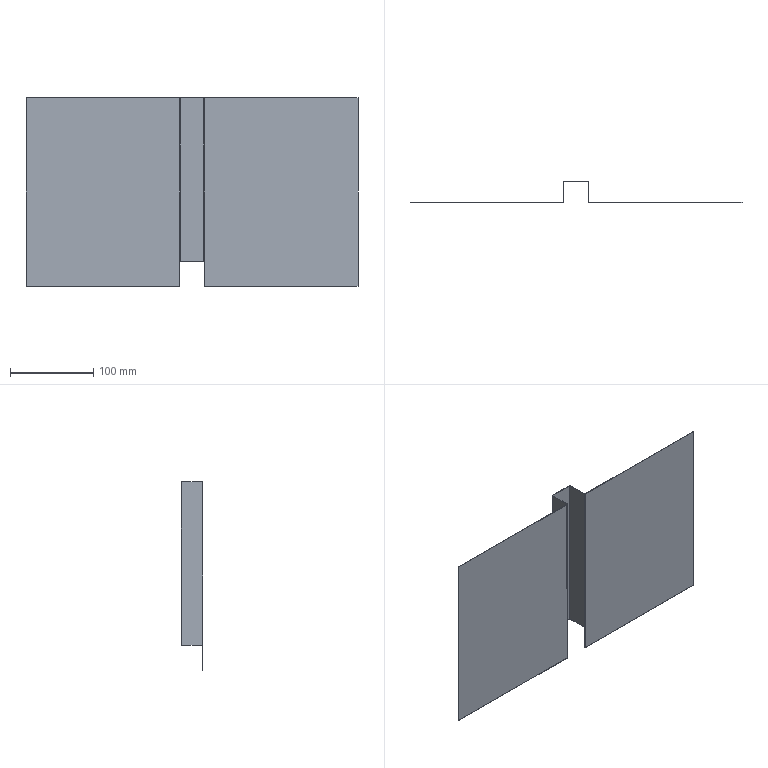Part | SolidWorks | features FlatPattern 1, ICE 1, SMBaseFlange 1, SheetMetal 1 | 1 solid | 36 faces | box 399 x 26 x 226 mm | volume 49527 mm3 | plane 28 | cylinder 8 | commonest cylinder face diameters 0.8 x4 1.8 x4
STEP:
#1=CARTESIAN_POINT('',(184.5,0.4,226.));
#2=VERTEX_POINT('',#1);
#3=CARTESIAN_POINT('',(185.,0.4,226.));
#4=VERTEX_POINT('',#3);
#5=CARTESIAN_POINT('',(184.5,0.4,226.));
#6=DIRECTION('',(1.,0.,0.));
#7=VECTOR('',#6,1000.);
#8=LINE('',#5,#7);
#9=EDGE_CURVE('',#2,#4,#8,.T.);
#10=ORIENTED_EDGE('',*,*,#9,.F.);
#11=CARTESIAN_POINT('',(184.1,0.,226.));
#12=VERTEX_POINT('',#11);
#13=CARTESIAN_POINT('',(184.1,0.4,226.));
#14=DIRECTION('',(0.,0.,1.));
#15=DIRECTION('',(-1.,0.,0.));
#16=AXIS2_PLACEMENT_3D('',#13,#14,#15);
#17=CIRCLE('',#16,0.4);
#18=EDGE_CURVE('',#12,#2,#17,.T.);
#19=ORIENTED_EDGE('',*,*,#18,.F.);
#20=CARTESIAN_POINT('',(184.1,-0.5,226.));
#21=VERTEX_POINT('',#20);
#22=CARTESIAN_POINT('',(184.1,-0.5,226.));
#23=DIRECTION('',(0.,1.,0.));
#24=VECTOR('',#23,1000.);
#25=LINE('',#22,#24);
#26=EDGE_CURVE('',#21,#12,#25,.T.);
#27=ORIENTED_EDGE('',*,*,#26,.F.);
#28=CARTESIAN_POINT('',(184.1,0.4,226.));
#29=DIRECTION('',(0.,0.,1.));
#30=DIRECTION('',(1.,0.,0.));
#31=AXIS2_PLACEMENT_3D('',#28,#29,#30);
#32=CIRCLE('',#31,0.9);
#33=EDGE_CURVE('',#21,#4,#32,.T.);
#34=ORIENTED_EDGE('',*,*,#33,.T.);
#35=EDGE_LOOP('',(#10,#19,#27,#34));
#36=FACE_OUTER_BOUND('',#35,.T.);
#37=CARTESIAN_POINT('',(184.5,0.4,226.));
#38=DIRECTION('',(0.,0.,1.));
#39=DIRECTION('',(1.,0.,0.));
#40=AXIS2_PLACEMENT_3D('',#37,#38,#39);
#41=PLANE('',#40);
#42=ADVANCED_FACE('',(#36),#41,.T.);
#43=CARTESIAN_POINT('',(184.5,24.6,226.));
#44=VERTEX_POINT('',#43);
#45=CARTESIAN_POINT('',(184.5,0.,226.));
#46=DIRECTION('',(0.,1.,0.));
#47=VECTOR('',#46,1000.);
#48=LINE('',#45,#47);
#49=EDGE_CURVE('',#2,#44,#48,.T.);
#50=ORIENTED_EDGE('',*,*,#49,.F.);
#51=ORIENTED_EDGE('',*,*,#9,.T.);
#52=CARTESIAN_POINT('',(185.,24.6,226.));
#53=VERTEX_POINT('',#52);
#54=CARTESIAN_POINT('',(185.,0.,226.));
#55=DIRECTION('',(0.,1.,0.));
#56=VECTOR('',#55,1000.);
#57=LINE('',#54,#56);
#58=EDGE_CURVE('',#4,#53,#57,.T.);
#59=ORIENTED_EDGE('',*,*,#58,.T.);
#60=CARTESIAN_POINT('',(185.,24.6,226.));
#61=DIRECTION('',(-1.,0.,0.));
#62=VECTOR('',#61,1000.);
#63=LINE('',#60,#62);
#64=EDGE_CURVE('',#53,#44,#63,.T.);
#65=ORIENTED_EDGE('',*,*,#64,.T.);
#66=EDGE_LOOP('',(#50,#51,#59,#65));
#67=FACE_OUTER_BOUND('',#66,.T.);
#68=CARTESIAN_POINT('',(184.1,-0.5,226.));
#69=DIRECTION('',(0.,0.,1.));
#70=DIRECTION('',(1.,0.,0.));
#71=AXIS2_PLACEMENT_3D('',#68,#69,#70);
#72=PLANE('',#71);
#73=ADVANCED_FACE('',(#67),#72,.T.);
#74=CARTESIAN_POINT('',(184.5,-0.4062,0.));
#75=VERTEX_POINT('',#74);
#76=CARTESIAN_POINT('',(184.5,0.4,0.));
#77=VERTEX_POINT('',#76);
#78=CARTESIAN_POINT('',(184.5,-0.501,0.));
#79=DIRECTION('',(0.,1.,0.));
#80=VECTOR('',#79,1000.);
#81=LINE('',#78,#80);
#82=EDGE_CURVE('',#75,#77,#81,.T.);
#83=ORIENTED_EDGE('',*,*,#82,.F.);
#84=CARTESIAN_POINT('',(184.1,-0.5,0.));
#85=VERTEX_POINT('',#84);
#86=CARTESIAN_POINT('',(184.1,0.4,0.));
#87=DIRECTION('',(0.,0.,1.));
#88=DIRECTION('',(1.,0.,0.));
#89=AXIS2_PLACEMENT_3D('',#86,#87,#88);
#90=CIRCLE('',#89,0.9);
#91=EDGE_CURVE('',#85,#75,#90,.T.);
#92=ORIENTED_EDGE('',*,*,#91,.F.);
#93=CARTESIAN_POINT('',(184.1,0.,0.));
#94=VERTEX_POINT('',#93);
#95=CARTESIAN_POINT('',(184.1,0.,0.));
#96=DIRECTION('',(0.,-1.,0.));
#97=VECTOR('',#96,1000.);
#98=LINE('',#95,#97);
#99=EDGE_CURVE('',#94,#85,#98,.T.);
#100=ORIENTED_EDGE('',*,*,#99,.F.);
#101=CARTESIAN_POINT('',(184.1,0.4,0.));
#102=DIRECTION('',(0.,0.,1.));
#103=DIRECTION('',(-1.,0.,0.));
#104=AXIS2_PLACEMENT_3D('',#101,#102,#103);
#105=CIRCLE('',#104,0.4);
#106=EDGE_CURVE('',#94,#77,#105,.T.);
#107=ORIENTED_EDGE('',*,*,#106,.T.);
#108=EDGE_LOOP('',(#83,#92,#100,#107));
#109=FACE_OUTER_BOUND('',#108,.T.);
#110=CARTESIAN_POINT('',(184.1,0.,0.));
#111=DIRECTION('',(0.,0.,-1.));
#112=DIRECTION('',(-1.,0.,0.));
#113=AXIS2_PLACEMENT_3D('',#110,#111,#112);
#114=PLANE('',#113);
#115=ADVANCED_FACE('',(#109),#114,.T.);
#116=CARTESIAN_POINT('',(0.,0.,0.));
#117=VERTEX_POINT('',#116);
#118=CARTESIAN_POINT('',(0.,0.,0.));
#119=DIRECTION('',(1.,0.,0.));
#120=VECTOR('',#119,1000.);
#121=LINE('',#118,#120);
#122=EDGE_CURVE('',#117,#94,#121,.T.);
#123=ORIENTED_EDGE('',*,*,#122,.T.);
#124=ORIENTED_EDGE('',*,*,#99,.T.);
#125=CARTESIAN_POINT('',(0.,-0.5,0.));
#126=VERTEX_POINT('',#125);
#127=CARTESIAN_POINT('',(0.,-0.5,0.));
#128=DIRECTION('',(1.,0.,0.));
#129=VECTOR('',#128,1000.);
#130=LINE('',#127,#129);
#131=EDGE_CURVE('',#126,#85,#130,.T.);
#132=ORIENTED_EDGE('',*,*,#131,.F.);
#133=CARTESIAN_POINT('',(0.,-0.5,0.));
#134=DIRECTION('',(0.,1.,0.));
#135=VECTOR('',#134,1000.);
#136=LINE('',#133,#135);
#137=EDGE_CURVE('',#126,#117,#136,.T.);
#138=ORIENTED_EDGE('',*,*,#137,.T.);
#139=EDGE_LOOP('',(#123,#124,#132,#138));
#140=FACE_OUTER_BOUND('',#139,.T.);
#141=CARTESIAN_POINT('',(185.,0.4,0.));
#142=DIRECTION('',(0.,0.,-1.));
#143=DIRECTION('',(-1.,0.,0.));
#144=AXIS2_PLACEMENT_3D('',#141,#142,#143);
#145=PLANE('',#144);
#146=ADVANCED_FACE('',(#140),#145,.T.);
#147=CARTESIAN_POINT('',(185.4,25.5,226.));
#148=VERTEX_POINT('',#147);
#149=CARTESIAN_POINT('',(185.4,25.,226.));
#150=VERTEX_POINT('',#149);
#151=CARTESIAN_POINT('',(185.4,25.5,226.));
#152=DIRECTION('',(0.,-1.,0.));
#153=VECTOR('',#152,1000.);
#154=LINE('',#151,#153);
#155=EDGE_CURVE('',#148,#150,#154,.T.);
#156=ORIENTED_EDGE('',*,*,#155,.F.);
#157=CARTESIAN_POINT('',(185.4,24.6,226.));
#158=DIRECTION('',(0.,0.,-1.));
#159=DIRECTION('',(1.,0.,0.));
#160=AXIS2_PLACEMENT_3D('',#157,#158,#159);
#161=CIRCLE('',#160,0.9);
#162=EDGE_CURVE('',#44,#148,#161,.T.);
#163=ORIENTED_EDGE('',*,*,#162,.F.);
#164=ORIENTED_EDGE('',*,*,#64,.F.);
#165=CARTESIAN_POINT('',(185.4,24.6,226.));
#166=DIRECTION('',(0.,0.,-1.));
#167=DIRECTION('',(1.,0.,0.));
#168=AXIS2_PLACEMENT_3D('',#165,#166,#167);
#169=CIRCLE('',#168,0.4);
#170=EDGE_CURVE('',#53,#150,#169,.T.);
#171=ORIENTED_EDGE('',*,*,#170,.T.);
#172=EDGE_LOOP('',(#156,#163,#164,#171));
#173=FACE_OUTER_BOUND('',#172,.T.);
#174=CARTESIAN_POINT('',(185.4,25.5,226.));
#175=DIRECTION('',(0.,0.,1.));
#176=DIRECTION('',(1.,0.,0.));
#177=AXIS2_PLACEMENT_3D('',#174,#175,#176);
#178=PLANE('',#177);
#179=ADVANCED_FACE('',(#173),#178,.T.);
#180=CARTESIAN_POINT('',(213.6,25.5,226.));
#181=VERTEX_POINT('',#180);
#182=CARTESIAN_POINT('',(184.5,25.5,226.));
#183=DIRECTION('',(1.,0.,0.));
#184=VECTOR('',#183,1000.);
#185=LINE('',#182,#184);
#186=EDGE_CURVE('',#148,#181,#185,.T.);
#187=ORIENTED_EDGE('',*,*,#186,.F.);
#188=ORIENTED_EDGE('',*,*,#155,.T.);
#189=CARTESIAN_POINT('',(213.6,25.,226.));
#190=VERTEX_POINT('',#189);
#191=CARTESIAN_POINT('',(184.5,25.,226.));
#192=DIRECTION('',(1.,0.,0.));
#193=VECTOR('',#192,1000.);
#194=LINE('',#191,#193);
#195=EDGE_CURVE('',#150,#190,#194,.T.);
#196=ORIENTED_EDGE('',*,*,#195,.T.);
#197=CARTESIAN_POINT('',(213.6,25.,226.));
#198=DIRECTION('',(0.,1.,0.));
#199=VECTOR('',#198,1000.);
#200=LINE('',#197,#199);
#201=EDGE_CURVE('',#190,#181,#200,.T.);
#202=ORIENTED_EDGE('',*,*,#201,.T.);
#203=EDGE_LOOP('',(#187,#188,#196,#202));
#204=FACE_OUTER_BOUND('',#203,.T.);
#205=CARTESIAN_POINT('',(185.,24.6,226.));
#206=DIRECTION('',(0.,0.,1.));
#207=DIRECTION('',(1.,0.,0.));
#208=AXIS2_PLACEMENT_3D('',#205,#206,#207);
#209=PLANE('',#208);
#210=ADVANCED_FACE('',(#204),#209,.T.);
#211=CARTESIAN_POINT('',(214.5,24.6,226.));
#212=VERTEX_POINT('',#211);
#213=CARTESIAN_POINT('',(214.,24.6,226.));
#214=VERTEX_POINT('',#213);
#215=CARTESIAN_POINT('',(214.5,24.6,226.));
#216=DIRECTION('',(-1.,0.,0.));
#217=VECTOR('',#216,1000.);
#218=LINE('',#215,#217);
#219=EDGE_CURVE('',#212,#214,#218,.T.);
#220=ORIENTED_EDGE('',*,*,#219,.F.);
#221=CARTESIAN_POINT('',(213.6,24.6,226.));
#222=DIRECTION('',(0.,0.,-1.));
#223=DIRECTION('',(1.,0.,0.));
#224=AXIS2_PLACEMENT_3D('',#221,#222,#223);
#225=CIRCLE('',#224,0.9);
#226=EDGE_CURVE('',#181,#212,#225,.T.);
#227=ORIENTED_EDGE('',*,*,#226,.F.);
#228=ORIENTED_EDGE('',*,*,#201,.F.);
#229=CARTESIAN_POINT('',(213.6,24.6,226.));
#230=DIRECTION('',(0.,0.,-1.));
#231=DIRECTION('',(1.,0.,0.));
#232=AXIS2_PLACEMENT_3D('',#229,#230,#231);
#233=CIRCLE('',#232,0.4);
#234=EDGE_CURVE('',#190,#214,#233,.T.);
#235=ORIENTED_EDGE('',*,*,#234,.T.);
#236=EDGE_LOOP('',(#220,#227,#228,#235));
#237=FACE_OUTER_BOUND('',#236,.T.);
#238=CARTESIAN_POINT('',(214.5,24.6,226.));
#239=DIRECTION('',(0.,0.,1.));
#240=DIRECTION('',(1.,0.,0.));
#241=AXIS2_PLACEMENT_3D('',#238,#239,#240);
#242=PLANE('',#241);
#243=ADVANCED_FACE('',(#237),#242,.T.);
#244=CARTESIAN_POINT('',(214.5,0.4,226.));
#245=VERTEX_POINT('',#244);
#246=CARTESIAN_POINT('',(214.5,25.5,226.));
#247=DIRECTION('',(0.,-1.,0.));
#248=VECTOR('',#247,1000.);
#249=LINE('',#246,#248);
#250=EDGE_CURVE('',#212,#245,#249,.T.);
#251=ORIENTED_EDGE('',*,*,#250,.F.);
#252=ORIENTED_EDGE('',*,*,#219,.T.);
#253=CARTESIAN_POINT('',(214.,0.4,226.));
#254=VERTEX_POINT('',#253);
#255=CARTESIAN_POINT('',(214.,25.5,226.));
#256=DIRECTION('',(0.,-1.,0.));
#257=VECTOR('',#256,1000.);
#258=LINE('',#255,#257);
#259=EDGE_CURVE('',#214,#254,#258,.T.);
#260=ORIENTED_EDGE('',*,*,#259,.T.);
#261=CARTESIAN_POINT('',(214.,0.4,226.));
#262=DIRECTION('',(1.,0.,0.));
#263=VECTOR('',#262,1000.);
#264=LINE('',#261,#263);
#265=EDGE_CURVE('',#254,#245,#264,.T.);
#266=ORIENTED_EDGE('',*,*,#265,.T.);
#267=EDGE_LOOP('',(#251,#252,#260,#266));
#268=FACE_OUTER_BOUND('',#267,.T.);
#269=CARTESIAN_POINT('',(213.6,25.,226.));
#270=DIRECTION('',(0.,0.,1.));
#271=DIRECTION('',(1.,0.,0.));
#272=AXIS2_PLACEMENT_3D('',#269,#270,#271);
#273=PLANE('',#272);
#274=ADVANCED_FACE('',(#268),#273,.T.);
#275=CARTESIAN_POINT('',(214.9,0.,226.));
#276=VERTEX_POINT('',#275);
#277=CARTESIAN_POINT('',(214.9,-0.5,226.));
#278=VERTEX_POINT('',#277);
#279=CARTESIAN_POINT('',(214.9,0.,226.));
#280=DIRECTION('',(0.,-1.,0.));
#281=VECTOR('',#280,1000.);
#282=LINE('',#279,#281);
#283=EDGE_CURVE('',#276,#278,#282,.T.);
#284=ORIENTED_EDGE('',*,*,#283,.F.);
#285=CARTESIAN_POINT('',(214.9,0.4,226.));
#286=DIRECTION('',(0.,0.,1.));
#287=DIRECTION('',(-1.,0.,0.));
#288=AXIS2_PLACEMENT_3D('',#285,#286,#287);
#289=CIRCLE('',#288,0.4);
#290=EDGE_CURVE('',#245,#276,#289,.T.);
#291=ORIENTED_EDGE('',*,*,#290,.F.);
#292=ORIENTED_EDGE('',*,*,#265,.F.);
#293=CARTESIAN_POINT('',(214.9,0.4,226.));
#294=DIRECTION('',(0.,0.,1.));
#295=DIRECTION('',(1.,0.,0.));
#296=AXIS2_PLACEMENT_3D('',#293,#294,#295);
#297=CIRCLE('',#296,0.9);
#298=EDGE_CURVE('',#254,#278,#297,.T.);
#299=ORIENTED_EDGE('',*,*,#298,.T.);
#300=EDGE_LOOP('',(#284,#291,#292,#299));
#301=FACE_OUTER_BOUND('',#300,.T.);
#302=CARTESIAN_POINT('',(214.9,0.,226.));
#303=DIRECTION('',(0.,0.,1.));
#304=DIRECTION('',(1.,0.,0.));
#305=AXIS2_PLACEMENT_3D('',#302,#303,#304);
#306=PLANE('',#305);
#307=ADVANCED_FACE('',(#301),#306,.T.);
#308=CARTESIAN_POINT('',(399.,0.,226.));
#309=VERTEX_POINT('',#308);
#310=CARTESIAN_POINT('',(214.5,0.,226.));
#311=DIRECTION('',(1.,0.,0.));
#312=VECTOR('',#311,1000.);
#313=LINE('',#310,#312);
#314=EDGE_CURVE('',#276,#309,#313,.T.);
#315=ORIENTED_EDGE('',*,*,#314,.F.);
#316=ORIENTED_EDGE('',*,*,#283,.T.);
#317=CARTESIAN_POINT('',(399.,-0.5,226.));
#318=VERTEX_POINT('',#317);
#319=CARTESIAN_POINT('',(214.5,-0.5,226.));
#320=DIRECTION('',(1.,0.,0.));
#321=VECTOR('',#320,1000.);
#322=LINE('',#319,#321);
#323=EDGE_CURVE('',#278,#318,#322,.T.);
#324=ORIENTED_EDGE('',*,*,#323,.T.);
#325=CARTESIAN_POINT('',(399.,0.,226.));
#326=DIRECTION('',(0.,-1.,0.));
#327=VECTOR('',#326,1000.);
#328=LINE('',#325,#327);
#329=EDGE_CURVE('',#309,#318,#328,.T.);
#330=ORIENTED_EDGE('',*,*,#329,.F.);
#331=EDGE_LOOP('',(#315,#316,#324,#330));
#332=FACE_OUTER_BOUND('',#331,.T.);
#333=CARTESIAN_POINT('',(214.,0.4,226.));
#334=DIRECTION('',(0.,0.,1.));
#335=DIRECTION('',(1.,0.,0.));
#336=AXIS2_PLACEMENT_3D('',#333,#334,#335);
#337=PLANE('',#336);
#338=ADVANCED_FACE('',(#332),#337,.T.);
#339=CARTESIAN_POINT('',(214.5,-0.4062,0.));
#340=VERTEX_POINT('',#339);
#341=CARTESIAN_POINT('',(214.5,0.4,0.));
#342=VERTEX_POINT('',#341);
#343=CARTESIAN_POINT('',(214.5,-0.501,0.));
#344=DIRECTION('',(0.,1.,0.));
#345=VECTOR('',#344,1000.);
#346=LINE('',#343,#345);
#347=EDGE_CURVE('',#340,#342,#346,.T.);
#348=ORIENTED_EDGE('',*,*,#347,.T.);
#349=CARTESIAN_POINT('',(214.9,0.,0.));
#350=VERTEX_POINT('',#349);
#351=CARTESIAN_POINT('',(214.9,0.4,0.));
#352=DIRECTION('',(0.,0.,1.));
#353=DIRECTION('',(-1.,0.,0.));
#354=AXIS2_PLACEMENT_3D('',#351,#352,#353);
#355=CIRCLE('',#354,0.4);
#356=EDGE_CURVE('',#342,#350,#355,.T.);
#357=ORIENTED_EDGE('',*,*,#356,.T.);
#358=CARTESIAN_POINT('',(214.9,-0.5,0.));
#359=VERTEX_POINT('',#358);
#360=CARTESIAN_POINT('',(214.9,-0.5,0.));
#361=DIRECTION('',(0.,1.,0.));
#362=VECTOR('',#361,1000.);
#363=LINE('',#360,#362);
#364=EDGE_CURVE('',#359,#350,#363,.T.);
#365=ORIENTED_EDGE('',*,*,#364,.F.);
#366=CARTESIAN_POINT('',(214.9,0.4,0.));
#367=DIRECTION('',(0.,0.,1.));
#368=DIRECTION('',(1.,0.,0.));
#369=AXIS2_PLACEMENT_3D('',#366,#367,#368);
#370=CIRCLE('',#369,0.9);
#371=EDGE_CURVE('',#340,#359,#370,.T.);
#372=ORIENTED_EDGE('',*,*,#371,.F.);
#373=EDGE_LOOP('',(#348,#357,#365,#372));
#374=FACE_OUTER_BOUND('',#373,.T.);
#375=CARTESIAN_POINT('',(214.5,0.4,0.));
#376=DIRECTION('',(0.,0.,-1.));
#377=DIRECTION('',(-1.,0.,0.));
#378=AXIS2_PLACEMENT_3D('',#375,#376,#377);
#379=PLANE('',#378);
#380=ADVANCED_FACE('',(#374),#379,.T.);
#381=CARTESIAN_POINT('',(399.,-0.5,0.));
#382=VERTEX_POINT('',#381);
#383=CARTESIAN_POINT('',(214.5,-0.5,0.));
#384=DIRECTION('',(1.,0.,0.));
#385=VECTOR('',#384,1000.);
#386=LINE('',#383,#385);
#387=EDGE_CURVE('',#359,#382,#386,.T.);
#388=ORIENTED_EDGE('',*,*,#387,.T.);
#389=CARTESIAN_POINT('',(399.,-0.5,226.));
#390=DIRECTION('',(0.,0.,-1.));
#391=VECTOR('',#390,1000.);
#392=LINE('',#389,#391);
#393=EDGE_CURVE('',#318,#382,#392,.T.);
#394=ORIENTED_EDGE('',*,*,#393,.F.);
#395=ORIENTED_EDGE('',*,*,#323,.F.);
#396=CARTESIAN_POINT('',(214.9,-0.5,226.));
#397=DIRECTION('',(0.,0.,-1.));
#398=VECTOR('',#397,1000.);
#399=LINE('',#396,#398);
#400=EDGE_CURVE('',#278,#359,#399,.T.);
#401=ORIENTED_EDGE('',*,*,#400,.T.);
#402=EDGE_LOOP('',(#388,#394,#395,#401));
#403=FACE_OUTER_BOUND('',#402,.T.);
#404=CARTESIAN_POINT('',(214.5,-0.5,226.));
#405=DIRECTION('',(0.,1.,0.));
#406=DIRECTION('',(0.,0.,1.));
#407=AXIS2_PLACEMENT_3D('',#404,#405,#406);
#408=PLANE('',#407);
#409=ADVANCED_FACE('',(#403),#408,.F.);
#410=CARTESIAN_POINT('',(399.,0.,0.));
#411=VERTEX_POINT('',#410);
#412=CARTESIAN_POINT('',(399.,0.,0.));
#413=DIRECTION('',(0.,-1.,0.));
#414=VECTOR('',#413,1000.);
#415=LINE('',#412,#414);
#416=EDGE_CURVE('',#411,#382,#415,.T.);
#417=ORIENTED_EDGE('',*,*,#416,.F.);
#418=CARTESIAN_POINT('',(399.,0.,226.));
#419=DIRECTION('',(0.,0.,-1.));
#420=VECTOR('',#419,1000.);
#421=LINE('',#418,#420);
#422=EDGE_CURVE('',#309,#411,#421,.T.);
#423=ORIENTED_EDGE('',*,*,#422,.F.);
#424=ORIENTED_EDGE('',*,*,#329,.T.);
#425=ORIENTED_EDGE('',*,*,#393,.T.);
#426=EDGE_LOOP('',(#417,#423,#424,#425));
#427=FACE_OUTER_BOUND('',#426,.T.);
#428=CARTESIAN_POINT('',(399.,0.,226.));
#429=DIRECTION('',(1.,0.,0.));
#430=DIRECTION('',(0.,0.,-1.));
#431=AXIS2_PLACEMENT_3D('',#428,#429,#430);
#432=PLANE('',#431);
#433=ADVANCED_FACE('',(#427),#432,.T.);
#434=CARTESIAN_POINT('',(214.5,0.,0.));
#435=DIRECTION('',(1.,0.,0.));
#436=VECTOR('',#435,1000.);
#437=LINE('',#434,#436);
#438=EDGE_CURVE('',#350,#411,#437,.T.);
#439=ORIENTED_EDGE('',*,*,#438,.F.);
#440=CARTESIAN_POINT('',(214.9,0.,226.));
#441=DIRECTION('',(0.,0.,-1.));
#442=VECTOR('',#441,1000.);
#443=LINE('',#440,#442);
#444=EDGE_CURVE('',#276,#350,#443,.T.);
#445=ORIENTED_EDGE('',*,*,#444,.F.);
#446=ORIENTED_EDGE('',*,*,#314,.T.);
#447=ORIENTED_EDGE('',*,*,#422,.T.);
#448=EDGE_LOOP('',(#439,#445,#446,#447));
#449=FACE_OUTER_BOUND('',#448,.T.);
#450=CARTESIAN_POINT('',(214.5,0.,226.));
#451=DIRECTION('',(0.,1.,0.));
#452=DIRECTION('',(0.,0.,1.));
#453=AXIS2_PLACEMENT_3D('',#450,#451,#452);
#454=PLANE('',#453);
#455=ADVANCED_FACE('',(#449),#454,.T.);
#456=ORIENTED_EDGE('',*,*,#356,.F.);
#457=CARTESIAN_POINT('',(214.5,0.4,30.));
#458=VERTEX_POINT('',#457);
#459=CARTESIAN_POINT('',(214.5,0.4,226.));
#460=DIRECTION('',(0.,0.,-1.));
#461=VECTOR('',#460,1000.);
#462=LINE('',#459,#461);
#463=EDGE_CURVE('',#458,#342,#462,.T.);
#464=ORIENTED_EDGE('',*,*,#463,.F.);
#465=CARTESIAN_POINT('',(214.5,0.4,226.));
#466=DIRECTION('',(0.,0.,-1.));
#467=VECTOR('',#466,1000.);
#468=LINE('',#465,#467);
#469=EDGE_CURVE('',#245,#458,#468,.T.);
#470=ORIENTED_EDGE('',*,*,#469,.F.);
#471=ORIENTED_EDGE('',*,*,#290,.T.);
#472=ORIENTED_EDGE('',*,*,#444,.T.);
#473=EDGE_LOOP('',(#456,#464,#470,#471,#472));
#474=FACE_OUTER_BOUND('',#473,.T.);
#475=CARTESIAN_POINT('',(214.9,0.4,226.));
#476=DIRECTION('',(0.,0.,-1.));
#477=DIRECTION('',(-1.,0.,0.));
#478=AXIS2_PLACEMENT_3D('',#475,#476,#477);
#479=CYLINDRICAL_SURFACE('',#478,0.4);
#480=ADVANCED_FACE('',(#474),#479,.F.);
#481=CARTESIAN_POINT('',(214.5,24.6,30.));
#482=VERTEX_POINT('',#481);
#483=CARTESIAN_POINT('',(214.5,-0.501,30.));
#484=DIRECTION('',(0.,1.,0.));
#485=VECTOR('',#484,1000.);
#486=LINE('',#483,#485);
#487=EDGE_CURVE('',#458,#482,#486,.T.);
#488=ORIENTED_EDGE('',*,*,#487,.T.);
#489=CARTESIAN_POINT('',(214.5,24.6,226.));
#490=DIRECTION('',(0.,0.,-1.));
#491=VECTOR('',#490,1000.);
#492=LINE('',#489,#491);
#493=EDGE_CURVE('',#212,#482,#492,.T.);
#494=ORIENTED_EDGE('',*,*,#493,.F.);
#495=ORIENTED_EDGE('',*,*,#250,.T.);
#496=ORIENTED_EDGE('',*,*,#469,.T.);
#497=EDGE_LOOP('',(#488,#494,#495,#496));
#498=FACE_OUTER_BOUND('',#497,.T.);
#499=CARTESIAN_POINT('',(214.5,25.5,226.));
#500=DIRECTION('',(1.,0.,0.));
#501=DIRECTION('',(0.,0.,-1.));
#502=AXIS2_PLACEMENT_3D('',#499,#500,#501);
#503=PLANE('',#502);
#504=ADVANCED_FACE('',(#498),#503,.T.);
#505=CARTESIAN_POINT('',(213.6,25.5,30.));
#506=VERTEX_POINT('',#505);
#507=CARTESIAN_POINT('',(213.6,24.6,30.));
#508=DIRECTION('',(0.,0.,1.));
#509=DIRECTION('',(1.,0.,0.));
#510=AXIS2_PLACEMENT_3D('',#507,#508,#509);
#511=CIRCLE('',#510,0.9);
#512=EDGE_CURVE('',#482,#506,#511,.T.);
#513=ORIENTED_EDGE('',*,*,#512,.T.);
#514=CARTESIAN_POINT('',(213.6,25.5,226.));
#515=DIRECTION('',(0.,0.,-1.));
#516=VECTOR('',#515,1000.);
#517=LINE('',#514,#516);
#518=EDGE_CURVE('',#181,#506,#517,.T.);
#519=ORIENTED_EDGE('',*,*,#518,.F.);
#520=ORIENTED_EDGE('',*,*,#226,.T.);
#521=ORIENTED_EDGE('',*,*,#493,.T.);
#522=EDGE_LOOP('',(#513,#519,#520,#521));
#523=FACE_OUTER_BOUND('',#522,.T.);
#524=CARTESIAN_POINT('',(213.6,24.6,226.));
#525=DIRECTION('',(0.,0.,-1.));
#526=DIRECTION('',(-1.,0.,0.));
#527=AXIS2_PLACEMENT_3D('',#524,#525,#526);
#528=CYLINDRICAL_SURFACE('',#527,0.9);
#529=ADVANCED_FACE('',(#523),#528,.T.);
#530=CARTESIAN_POINT('',(185.4,25.5,30.));
#531=VERTEX_POINT('',#530);
#532=CARTESIAN_POINT('',(184.5,25.5,30.));
#533=DIRECTION('',(1.,0.,0.));
#534=VECTOR('',#533,1000.);
#535=LINE('',#532,#534);
#536=EDGE_CURVE('',#531,#506,#535,.T.);
#537=ORIENTED_EDGE('',*,*,#536,.F.);
#538=CARTESIAN_POINT('',(185.4,25.5,226.));
#539=DIRECTION('',(0.,0.,-1.));
#540=VECTOR('',#539,1000.);
#541=LINE('',#538,#540);
#542=EDGE_CURVE('',#148,#531,#541,.T.);
#543=ORIENTED_EDGE('',*,*,#542,.F.);
#544=ORIENTED_EDGE('',*,*,#186,.T.);
#545=ORIENTED_EDGE('',*,*,#518,.T.);
#546=EDGE_LOOP('',(#537,#543,#544,#545));
#547=FACE_OUTER_BOUND('',#546,.T.);
#548=CARTESIAN_POINT('',(184.5,25.5,226.));
#549=DIRECTION('',(0.,1.,0.));
#550=DIRECTION('',(0.,0.,1.));
#551=AXIS2_PLACEMENT_3D('',#548,#549,#550);
#552=PLANE('',#551);
#553=ADVANCED_FACE('',(#547),#552,.T.);
#554=CARTESIAN_POINT('',(184.5,24.6,30.));
#555=VERTEX_POINT('',#554);
#556=CARTESIAN_POINT('',(185.4,24.6,30.));
#557=DIRECTION('',(0.,0.,1.));
#558=DIRECTION('',(1.,0.,0.));
#559=AXIS2_PLACEMENT_3D('',#556,#557,#558);
#560=CIRCLE('',#559,0.9);
#561=EDGE_CURVE('',#531,#555,#560,.T.);
#562=ORIENTED_EDGE('',*,*,#561,.T.);
#563=CARTESIAN_POINT('',(184.5,24.6,226.));
#564=DIRECTION('',(0.,0.,-1.));
#565=VECTOR('',#564,1000.);
#566=LINE('',#563,#565);
#567=EDGE_CURVE('',#44,#555,#566,.T.);
#568=ORIENTED_EDGE('',*,*,#567,.F.);
#569=ORIENTED_EDGE('',*,*,#162,.T.);
#570=ORIENTED_EDGE('',*,*,#542,.T.);
#571=EDGE_LOOP('',(#562,#568,#569,#570));
#572=FACE_OUTER_BOUND('',#571,.T.);
#573=CARTESIAN_POINT('',(185.4,24.6,226.));
#574=DIRECTION('',(0.,0.,-1.));
#575=DIRECTION('',(-1.,0.,0.));
#576=AXIS2_PLACEMENT_3D('',#573,#574,#575);
#577=CYLINDRICAL_SURFACE('',#576,0.9);
#578=ADVANCED_FACE('',(#572),#577,.T.);
#579=CARTESIAN_POINT('',(184.5,0.4,30.));
#580=VERTEX_POINT('',#579);
#581=CARTESIAN_POINT('',(184.5,-0.501,30.));
#582=DIRECTION('',(0.,1.,0.));
#583=VECTOR('',#582,1000.);
#584=LINE('',#581,#583);
#585=EDGE_CURVE('',#580,#555,#584,.T.);
#586=ORIENTED_EDGE('',*,*,#585,.F.);
#587=CARTESIAN_POINT('',(184.5,0.4,226.));
#588=DIRECTION('',(0.,0.,-1.));
#589=VECTOR('',#588,1000.);
#590=LINE('',#587,#589);
#591=EDGE_CURVE('',#2,#580,#590,.T.);
#592=ORIENTED_EDGE('',*,*,#591,.F.);
#593=ORIENTED_EDGE('',*,*,#49,.T.);
#594=ORIENTED_EDGE('',*,*,#567,.T.);
#595=EDGE_LOOP('',(#586,#592,#593,#594));
#596=FACE_OUTER_BOUND('',#595,.T.);
#597=CARTESIAN_POINT('',(184.5,0.,226.));
#598=DIRECTION('',(-1.,0.,0.));
#599=DIRECTION('',(0.,0.,1.));
#600=AXIS2_PLACEMENT_3D('',#597,#598,#599);
#601=PLANE('',#600);
#602=ADVANCED_FACE('',(#596),#601,.T.);
#603=ORIENTED_EDGE('',*,*,#106,.F.);
#604=CARTESIAN_POINT('',(184.1,0.,226.));
#605=DIRECTION('',(0.,0.,-1.));
#606=VECTOR('',#605,1000.);
#607=LINE('',#604,#606);
#608=EDGE_CURVE('',#12,#94,#607,.T.);
#609=ORIENTED_EDGE('',*,*,#608,.F.);
#610=ORIENTED_EDGE('',*,*,#18,.T.);
#611=ORIENTED_EDGE('',*,*,#591,.T.);
#612=CARTESIAN_POINT('',(184.5,0.4,226.));
#613=DIRECTION('',(0.,0.,-1.));
#614=VECTOR('',#613,1000.);
#615=LINE('',#612,#614);
#616=EDGE_CURVE('',#580,#77,#615,.T.);
#617=ORIENTED_EDGE('',*,*,#616,.T.);
#618=EDGE_LOOP('',(#603,#609,#610,#611,#617));
#619=FACE_OUTER_BOUND('',#618,.T.);
#620=CARTESIAN_POINT('',(184.1,0.4,226.));
#621=DIRECTION('',(0.,0.,-1.));
#622=DIRECTION('',(-1.,0.,0.));
#623=AXIS2_PLACEMENT_3D('',#620,#621,#622);
#624=CYLINDRICAL_SURFACE('',#623,0.4);
#625=ADVANCED_FACE('',(#619),#624,.F.);
#626=ORIENTED_EDGE('',*,*,#122,.F.);
#627=CARTESIAN_POINT('',(0.,0.,226.));
#628=VERTEX_POINT('',#627);
#629=CARTESIAN_POINT('',(0.,0.,226.));
#630=DIRECTION('',(0.,0.,-1.));
#631=VECTOR('',#630,1000.);
#632=LINE('',#629,#631);
#633=EDGE_CURVE('',#628,#117,#632,.T.);
#634=ORIENTED_EDGE('',*,*,#633,.F.);
#635=CARTESIAN_POINT('',(0.,0.,226.));
#636=DIRECTION('',(1.,0.,0.));
#637=VECTOR('',#636,1000.);
#638=LINE('',#635,#637);
#639=EDGE_CURVE('',#628,#12,#638,.T.);
#640=ORIENTED_EDGE('',*,*,#639,.T.);
#641=ORIENTED_EDGE('',*,*,#608,.T.);
#642=EDGE_LOOP('',(#626,#634,#640,#641));
#643=FACE_OUTER_BOUND('',#642,.T.);
#644=CARTESIAN_POINT('',(0.,0.,226.));
#645=DIRECTION('',(0.,1.,0.));
#646=DIRECTION('',(0.,0.,1.));
#647=AXIS2_PLACEMENT_3D('',#644,#645,#646);
#648=PLANE('',#647);
#649=ADVANCED_FACE('',(#643),#648,.T.);
#650=ORIENTED_EDGE('',*,*,#137,.F.);
#651=CARTESIAN_POINT('',(0.,-0.5,226.));
#652=VERTEX_POINT('',#651);
#653=CARTESIAN_POINT('',(0.,-0.5,226.));
#654=DIRECTION('',(0.,0.,-1.));
#655=VECTOR('',#654,1000.);
#656=LINE('',#653,#655);
#657=EDGE_CURVE('',#652,#126,#656,.T.);
#658=ORIENTED_EDGE('',*,*,#657,.F.);
#659=CARTESIAN_POINT('',(0.,-0.5,226.));
#660=DIRECTION('',(0.,1.,0.));
#661=VECTOR('',#660,1000.);
#662=LINE('',#659,#661);
#663=EDGE_CURVE('',#652,#628,#662,.T.);
#664=ORIENTED_EDGE('',*,*,#663,.T.);
#665=ORIENTED_EDGE('',*,*,#633,.T.);
#666=EDGE_LOOP('',(#650,#658,#664,#665));
#667=FACE_OUTER_BOUND('',#666,.T.);
#668=CARTESIAN_POINT('',(0.,-0.5,226.));
#669=DIRECTION('',(-1.,0.,0.));
#670=DIRECTION('',(0.,0.,1.));
#671=AXIS2_PLACEMENT_3D('',#668,#669,#670);
#672=PLANE('',#671);
#673=ADVANCED_FACE('',(#667),#672,.T.);
#674=ORIENTED_EDGE('',*,*,#131,.T.);
#675=CARTESIAN_POINT('',(184.1,-0.5,226.));
#676=DIRECTION('',(0.,0.,-1.));
#677=VECTOR('',#676,1000.);
#678=LINE('',#675,#677);
#679=EDGE_CURVE('',#21,#85,#678,.T.);
#680=ORIENTED_EDGE('',*,*,#679,.F.);
#681=CARTESIAN_POINT('',(0.,-0.5,226.));
#682=DIRECTION('',(1.,0.,0.));
#683=VECTOR('',#682,1000.);
#684=LINE('',#681,#683);
#685=EDGE_CURVE('',#652,#21,#684,.T.);
#686=ORIENTED_EDGE('',*,*,#685,.F.);
#687=ORIENTED_EDGE('',*,*,#657,.T.);
#688=EDGE_LOOP('',(#674,#680,#686,#687));
#689=FACE_OUTER_BOUND('',#688,.T.);
#690=CARTESIAN_POINT('',(0.,-0.5,226.));
#691=DIRECTION('',(0.,1.,0.));
#692=DIRECTION('',(0.,0.,1.));
#693=AXIS2_PLACEMENT_3D('',#690,#691,#692);
#694=PLANE('',#693);
#695=ADVANCED_FACE('',(#689),#694,.F.);
#696=ORIENTED_EDGE('',*,*,#91,.T.);
#697=CARTESIAN_POINT('',(184.5,-0.4062,30.));
#698=VERTEX_POINT('',#697);
#699=CARTESIAN_POINT('',(184.5,-0.4062,226.));
#700=DIRECTION('',(0.,0.,-1.));
#701=VECTOR('',#700,1000.);
#702=LINE('',#699,#701);
#703=EDGE_CURVE('',#698,#75,#702,.T.);
#704=ORIENTED_EDGE('',*,*,#703,.F.);
#705=CARTESIAN_POINT('',(185.,0.4,30.));
#706=VERTEX_POINT('',#705);
#707=CARTESIAN_POINT('',(184.1,0.4,30.));
#708=DIRECTION('',(0.,0.,-1.));
#709=DIRECTION('',(1.,0.,0.));
#710=AXIS2_PLACEMENT_3D('',#707,#708,#709);
#711=CIRCLE('',#710,0.9);
#712=EDGE_CURVE('',#706,#698,#711,.T.);
#713=ORIENTED_EDGE('',*,*,#712,.F.);
#714=CARTESIAN_POINT('',(185.,0.4,226.));
#715=DIRECTION('',(0.,0.,-1.));
#716=VECTOR('',#715,1000.);
#717=LINE('',#714,#716);
#718=EDGE_CURVE('',#4,#706,#717,.T.);
#719=ORIENTED_EDGE('',*,*,#718,.F.);
#720=ORIENTED_EDGE('',*,*,#33,.F.);
#721=ORIENTED_EDGE('',*,*,#679,.T.);
#722=EDGE_LOOP('',(#696,#704,#713,#719,#720,#721));
#723=FACE_OUTER_BOUND('',#722,.T.);
#724=CARTESIAN_POINT('',(184.1,0.4,226.));
#725=DIRECTION('',(0.,0.,-1.));
#726=DIRECTION('',(-1.,0.,0.));
#727=AXIS2_PLACEMENT_3D('',#724,#725,#726);
#728=CYLINDRICAL_SURFACE('',#727,0.9);
#729=ADVANCED_FACE('',(#723),#728,.T.);
#730=ORIENTED_EDGE('',*,*,#718,.T.);
#731=CARTESIAN_POINT('',(185.,24.6,30.));
#732=VERTEX_POINT('',#731);
#733=CARTESIAN_POINT('',(185.,-0.501,30.));
#734=DIRECTION('',(0.,-1.,0.));
#735=VECTOR('',#734,1000.);
#736=LINE('',#733,#735);
#737=EDGE_CURVE('',#732,#706,#736,.T.);
#738=ORIENTED_EDGE('',*,*,#737,.F.);
#739=CARTESIAN_POINT('',(185.,24.6,226.));
#740=DIRECTION('',(0.,0.,-1.));
#741=VECTOR('',#740,1000.);
#742=LINE('',#739,#741);
#743=EDGE_CURVE('',#53,#732,#742,.T.);
#744=ORIENTED_EDGE('',*,*,#743,.F.);
#745=ORIENTED_EDGE('',*,*,#58,.F.);
#746=EDGE_LOOP('',(#730,#738,#744,#745));
#747=FACE_OUTER_BOUND('',#746,.T.);
#748=CARTESIAN_POINT('',(185.,0.,226.));
#749=DIRECTION('',(-1.,0.,0.));
#750=DIRECTION('',(0.,0.,1.));
#751=AXIS2_PLACEMENT_3D('',#748,#749,#750);
#752=PLANE('',#751);
#753=ADVANCED_FACE('',(#747),#752,.F.);
#754=ORIENTED_EDGE('',*,*,#743,.T.);
#755=CARTESIAN_POINT('',(185.4,25.,30.));
#756=VERTEX_POINT('',#755);
#757=CARTESIAN_POINT('',(185.4,24.6,30.));
#758=DIRECTION('',(0.,0.,1.));
#759=DIRECTION('',(1.,0.,0.));
#760=AXIS2_PLACEMENT_3D('',#757,#758,#759);
#761=CIRCLE('',#760,0.4);
#762=EDGE_CURVE('',#756,#732,#761,.T.);
#763=ORIENTED_EDGE('',*,*,#762,.F.);
#764=CARTESIAN_POINT('',(185.4,25.,226.));
#765=DIRECTION('',(0.,0.,-1.));
#766=VECTOR('',#765,1000.);
#767=LINE('',#764,#766);
#768=EDGE_CURVE('',#150,#756,#767,.T.);
#769=ORIENTED_EDGE('',*,*,#768,.F.);
#770=ORIENTED_EDGE('',*,*,#170,.F.);
#771=EDGE_LOOP('',(#754,#763,#769,#770));
#772=FACE_OUTER_BOUND('',#771,.T.);
#773=CARTESIAN_POINT('',(185.4,24.6,226.));
#774=DIRECTION('',(0.,0.,-1.));
#775=DIRECTION('',(-1.,0.,0.));
#776=AXIS2_PLACEMENT_3D('',#773,#774,#775);
#777=CYLINDRICAL_SURFACE('',#776,0.4);
#778=ADVANCED_FACE('',(#772),#777,.F.);
#779=ORIENTED_EDGE('',*,*,#768,.T.);
#780=CARTESIAN_POINT('',(213.6,25.,30.));
#781=VERTEX_POINT('',#780);
#782=CARTESIAN_POINT('',(184.5,25.,30.));
#783=DIRECTION('',(-1.,0.,0.));
#784=VECTOR('',#783,1000.);
#785=LINE('',#782,#784);
#786=EDGE_CURVE('',#781,#756,#785,.T.);
#787=ORIENTED_EDGE('',*,*,#786,.F.);
#788=CARTESIAN_POINT('',(213.6,25.,226.));
#789=DIRECTION('',(0.,0.,-1.));
#790=VECTOR('',#789,1000.);
#791=LINE('',#788,#790);
#792=EDGE_CURVE('',#190,#781,#791,.T.);
#793=ORIENTED_EDGE('',*,*,#792,.F.);
#794=ORIENTED_EDGE('',*,*,#195,.F.);
#795=EDGE_LOOP('',(#779,#787,#793,#794));
#796=FACE_OUTER_BOUND('',#795,.T.);
#797=CARTESIAN_POINT('',(184.5,25.,226.));
#798=DIRECTION('',(0.,1.,0.));
#799=DIRECTION('',(0.,0.,1.));
#800=AXIS2_PLACEMENT_3D('',#797,#798,#799);
#801=PLANE('',#800);
#802=ADVANCED_FACE('',(#796),#801,.F.);
#803=ORIENTED_EDGE('',*,*,#792,.T.);
#804=CARTESIAN_POINT('',(214.,24.6,30.));
#805=VERTEX_POINT('',#804);
#806=CARTESIAN_POINT('',(213.6,24.6,30.));
#807=DIRECTION('',(0.,0.,1.));
#808=DIRECTION('',(1.,0.,0.));
#809=AXIS2_PLACEMENT_3D('',#806,#807,#808);
#810=CIRCLE('',#809,0.4);
#811=EDGE_CURVE('',#805,#781,#810,.T.);
#812=ORIENTED_EDGE('',*,*,#811,.F.);
#813=CARTESIAN_POINT('',(214.,24.6,226.));
#814=DIRECTION('',(0.,0.,-1.));
#815=VECTOR('',#814,1000.);
#816=LINE('',#813,#815);
#817=EDGE_CURVE('',#214,#805,#816,.T.);
#818=ORIENTED_EDGE('',*,*,#817,.F.);
#819=ORIENTED_EDGE('',*,*,#234,.F.);
#820=EDGE_LOOP('',(#803,#812,#818,#819));
#821=FACE_OUTER_BOUND('',#820,.T.);
#822=CARTESIAN_POINT('',(213.6,24.6,226.));
#823=DIRECTION('',(0.,0.,-1.));
#824=DIRECTION('',(-1.,0.,0.));
#825=AXIS2_PLACEMENT_3D('',#822,#823,#824);
#826=CYLINDRICAL_SURFACE('',#825,0.4);
#827=ADVANCED_FACE('',(#821),#826,.F.);
#828=ORIENTED_EDGE('',*,*,#817,.T.);
#829=CARTESIAN_POINT('',(214.,0.4,30.));
#830=VERTEX_POINT('',#829);
#831=CARTESIAN_POINT('',(214.,-0.501,30.));
#832=DIRECTION('',(0.,1.,0.));
#833=VECTOR('',#832,1000.);
#834=LINE('',#831,#833);
#835=EDGE_CURVE('',#830,#805,#834,.T.);
#836=ORIENTED_EDGE('',*,*,#835,.F.);
#837=CARTESIAN_POINT('',(214.,0.4,226.));
#838=DIRECTION('',(0.,0.,-1.));
#839=VECTOR('',#838,1000.);
#840=LINE('',#837,#839);
#841=EDGE_CURVE('',#254,#830,#840,.T.);
#842=ORIENTED_EDGE('',*,*,#841,.F.);
#843=ORIENTED_EDGE('',*,*,#259,.F.);
#844=EDGE_LOOP('',(#828,#836,#842,#843));
#845=FACE_OUTER_BOUND('',#844,.T.);
#846=CARTESIAN_POINT('',(214.,25.5,226.));
#847=DIRECTION('',(1.,0.,0.));
#848=DIRECTION('',(0.,0.,-1.));
#849=AXIS2_PLACEMENT_3D('',#846,#847,#848);
#850=PLANE('',#849);
#851=ADVANCED_FACE('',(#845),#850,.F.);
#852=CARTESIAN_POINT('',(214.5,-0.4062,30.));
#853=VERTEX_POINT('',#852);
#854=CARTESIAN_POINT('',(214.9,0.4,30.));
#855=DIRECTION('',(0.,0.,-1.));
#856=DIRECTION('',(1.,0.,0.));
#857=AXIS2_PLACEMENT_3D('',#854,#855,#856);
#858=CIRCLE('',#857,0.9);
#859=EDGE_CURVE('',#853,#830,#858,.T.);
#860=ORIENTED_EDGE('',*,*,#859,.F.);
#861=CARTESIAN_POINT('',(214.5,-0.4062,226.));
#862=DIRECTION('',(0.,0.,1.));
#863=VECTOR('',#862,1000.);
#864=LINE('',#861,#863);
#865=EDGE_CURVE('',#340,#853,#864,.T.);
#866=ORIENTED_EDGE('',*,*,#865,.F.);
#867=ORIENTED_EDGE('',*,*,#371,.T.);
#868=ORIENTED_EDGE('',*,*,#400,.F.);
#869=ORIENTED_EDGE('',*,*,#298,.F.);
#870=ORIENTED_EDGE('',*,*,#841,.T.);
#871=EDGE_LOOP('',(#860,#866,#867,#868,#869,#870));
#872=FACE_OUTER_BOUND('',#871,.T.);
#873=CARTESIAN_POINT('',(214.9,0.4,226.));
#874=DIRECTION('',(0.,0.,-1.));
#875=DIRECTION('',(-1.,0.,0.));
#876=AXIS2_PLACEMENT_3D('',#873,#874,#875);
#877=CYLINDRICAL_SURFACE('',#876,0.9);
#878=ADVANCED_FACE('',(#872),#877,.T.);
#879=ORIENTED_EDGE('',*,*,#685,.T.);
#880=ORIENTED_EDGE('',*,*,#26,.T.);
#881=ORIENTED_EDGE('',*,*,#639,.F.);
#882=ORIENTED_EDGE('',*,*,#663,.F.);
#883=EDGE_LOOP('',(#879,#880,#881,#882));
#884=FACE_OUTER_BOUND('',#883,.T.);
#885=CARTESIAN_POINT('',(214.9,0.4,226.));
#886=DIRECTION('',(0.,0.,-1.));
#887=DIRECTION('',(-1.,0.,0.));
#888=AXIS2_PLACEMENT_3D('',#885,#886,#887);
#889=PLANE('',#888);
#890=ADVANCED_FACE('',(#884),#889,.F.);
#891=ORIENTED_EDGE('',*,*,#387,.F.);
#892=ORIENTED_EDGE('',*,*,#364,.T.);
#893=ORIENTED_EDGE('',*,*,#438,.T.);
#894=ORIENTED_EDGE('',*,*,#416,.T.);
#895=EDGE_LOOP('',(#891,#892,#893,#894));
#896=FACE_OUTER_BOUND('',#895,.T.);
#897=CARTESIAN_POINT('',(214.9,0.4,0.));
#898=DIRECTION('',(0.,0.,-1.));
#899=DIRECTION('',(-1.,0.,0.));
#900=AXIS2_PLACEMENT_3D('',#897,#898,#899);
#901=PLANE('',#900);
#902=ADVANCED_FACE('',(#896),#901,.T.);
#903=CARTESIAN_POINT('',(184.5,-0.501,30.));
#904=DIRECTION('',(0.,1.,0.));
#905=VECTOR('',#904,1000.);
#906=LINE('',#903,#905);
#907=EDGE_CURVE('',#698,#580,#906,.T.);
#908=ORIENTED_EDGE('',*,*,#907,.F.);
#909=ORIENTED_EDGE('',*,*,#703,.T.);
#910=ORIENTED_EDGE('',*,*,#82,.T.);
#911=ORIENTED_EDGE('',*,*,#616,.F.);
#912=EDGE_LOOP('',(#908,#909,#910,#911));
#913=FACE_OUTER_BOUND('',#912,.T.);
#914=CARTESIAN_POINT('',(184.5,-0.501,0.));
#915=DIRECTION('',(-1.,0.,0.));
#916=DIRECTION('',(0.,0.,1.));
#917=AXIS2_PLACEMENT_3D('',#914,#915,#916);
#918=PLANE('',#917);
#919=ADVANCED_FACE('',(#913),#918,.F.);
#920=ORIENTED_EDGE('',*,*,#463,.T.);
#921=ORIENTED_EDGE('',*,*,#347,.F.);
#922=ORIENTED_EDGE('',*,*,#865,.T.);
#923=CARTESIAN_POINT('',(214.5,-0.501,30.));
#924=DIRECTION('',(0.,1.,0.));
#925=VECTOR('',#924,1000.);
#926=LINE('',#923,#925);
#927=EDGE_CURVE('',#853,#458,#926,.T.);
#928=ORIENTED_EDGE('',*,*,#927,.T.);
#929=EDGE_LOOP('',(#920,#921,#922,#928));
#930=FACE_OUTER_BOUND('',#929,.T.);
#931=CARTESIAN_POINT('',(214.5,-0.501,0.));
#932=DIRECTION('',(1.,0.,0.));
#933=DIRECTION('',(0.,0.,-1.));
#934=AXIS2_PLACEMENT_3D('',#931,#932,#933);
#935=PLANE('',#934);
#936=ADVANCED_FACE('',(#930),#935,.F.);
#937=ORIENTED_EDGE('',*,*,#927,.F.);
#938=ORIENTED_EDGE('',*,*,#859,.T.);
#939=ORIENTED_EDGE('',*,*,#835,.T.);
#940=ORIENTED_EDGE('',*,*,#811,.T.);
#941=ORIENTED_EDGE('',*,*,#786,.T.);
#942=ORIENTED_EDGE('',*,*,#762,.T.);
#943=ORIENTED_EDGE('',*,*,#737,.T.);
#944=ORIENTED_EDGE('',*,*,#712,.T.);
#945=ORIENTED_EDGE('',*,*,#907,.T.);
#946=ORIENTED_EDGE('',*,*,#585,.T.);
#947=ORIENTED_EDGE('',*,*,#561,.F.);
#948=ORIENTED_EDGE('',*,*,#536,.T.);
#949=ORIENTED_EDGE('',*,*,#512,.F.);
#950=ORIENTED_EDGE('',*,*,#487,.F.);
#951=EDGE_LOOP('',(#937,#938,#939,#940,#941,#942,#943,#944,#945,#946,#947,#948,#949,#950));
#952=FACE_OUTER_BOUND('',#951,.T.);
#953=CARTESIAN_POINT('',(184.5,-0.501,30.));
#954=DIRECTION('',(0.,0.,1.));
#955=DIRECTION('',(1.,0.,0.));
#956=AXIS2_PLACEMENT_3D('',#953,#954,#955);
#957=PLANE('',#956);
#958=ADVANCED_FACE('',(#952),#957,.F.);
#959=CLOSED_SHELL('',(#42,#73,#115,#146,#179,#210,#243,#274,#307,#338,#380,#409,#433,#455,#480,#504,#529,#553,#578,#602,#625,#649,#673,#695,#729,#753,#778,#802,#827,#851,#878,#890,#902,#919,#936,#958));
#960=MANIFOLD_SOLID_BREP('',#959);
#961=CARTESIAN_POINT('',(0.,0.,0.));
#962=DIRECTION('',(0.,0.,1.));
#963=DIRECTION('',(1.,0.,0.));
#964=AXIS2_PLACEMENT_3D('',#961,#962,#963);
#965=(LENGTH_UNIT()NAMED_UNIT(*)SI_UNIT(.MILLI.,.METRE.));
#966=UNCERTAINTY_MEASURE_WITH_UNIT(LENGTH_MEASURE(0.00001),#965,'','');
#967=(NAMED_UNIT(*)PLANE_ANGLE_UNIT()SI_UNIT($,.RADIAN.));
#968=(NAMED_UNIT(*)SI_UNIT($,.STERADIAN.)SOLID_ANGLE_UNIT());
#969=(GEOMETRIC_REPRESENTATION_CONTEXT(3)GLOBAL_UNCERTAINTY_ASSIGNED_CONTEXT((#966))GLOBAL_UNIT_ASSIGNED_CONTEXT((#965,#967,#968))REPRESENTATION_CONTEXT('',''));
#970=ADVANCED_BREP_SHAPE_REPRESENTATION('',(#960,#964),#969);